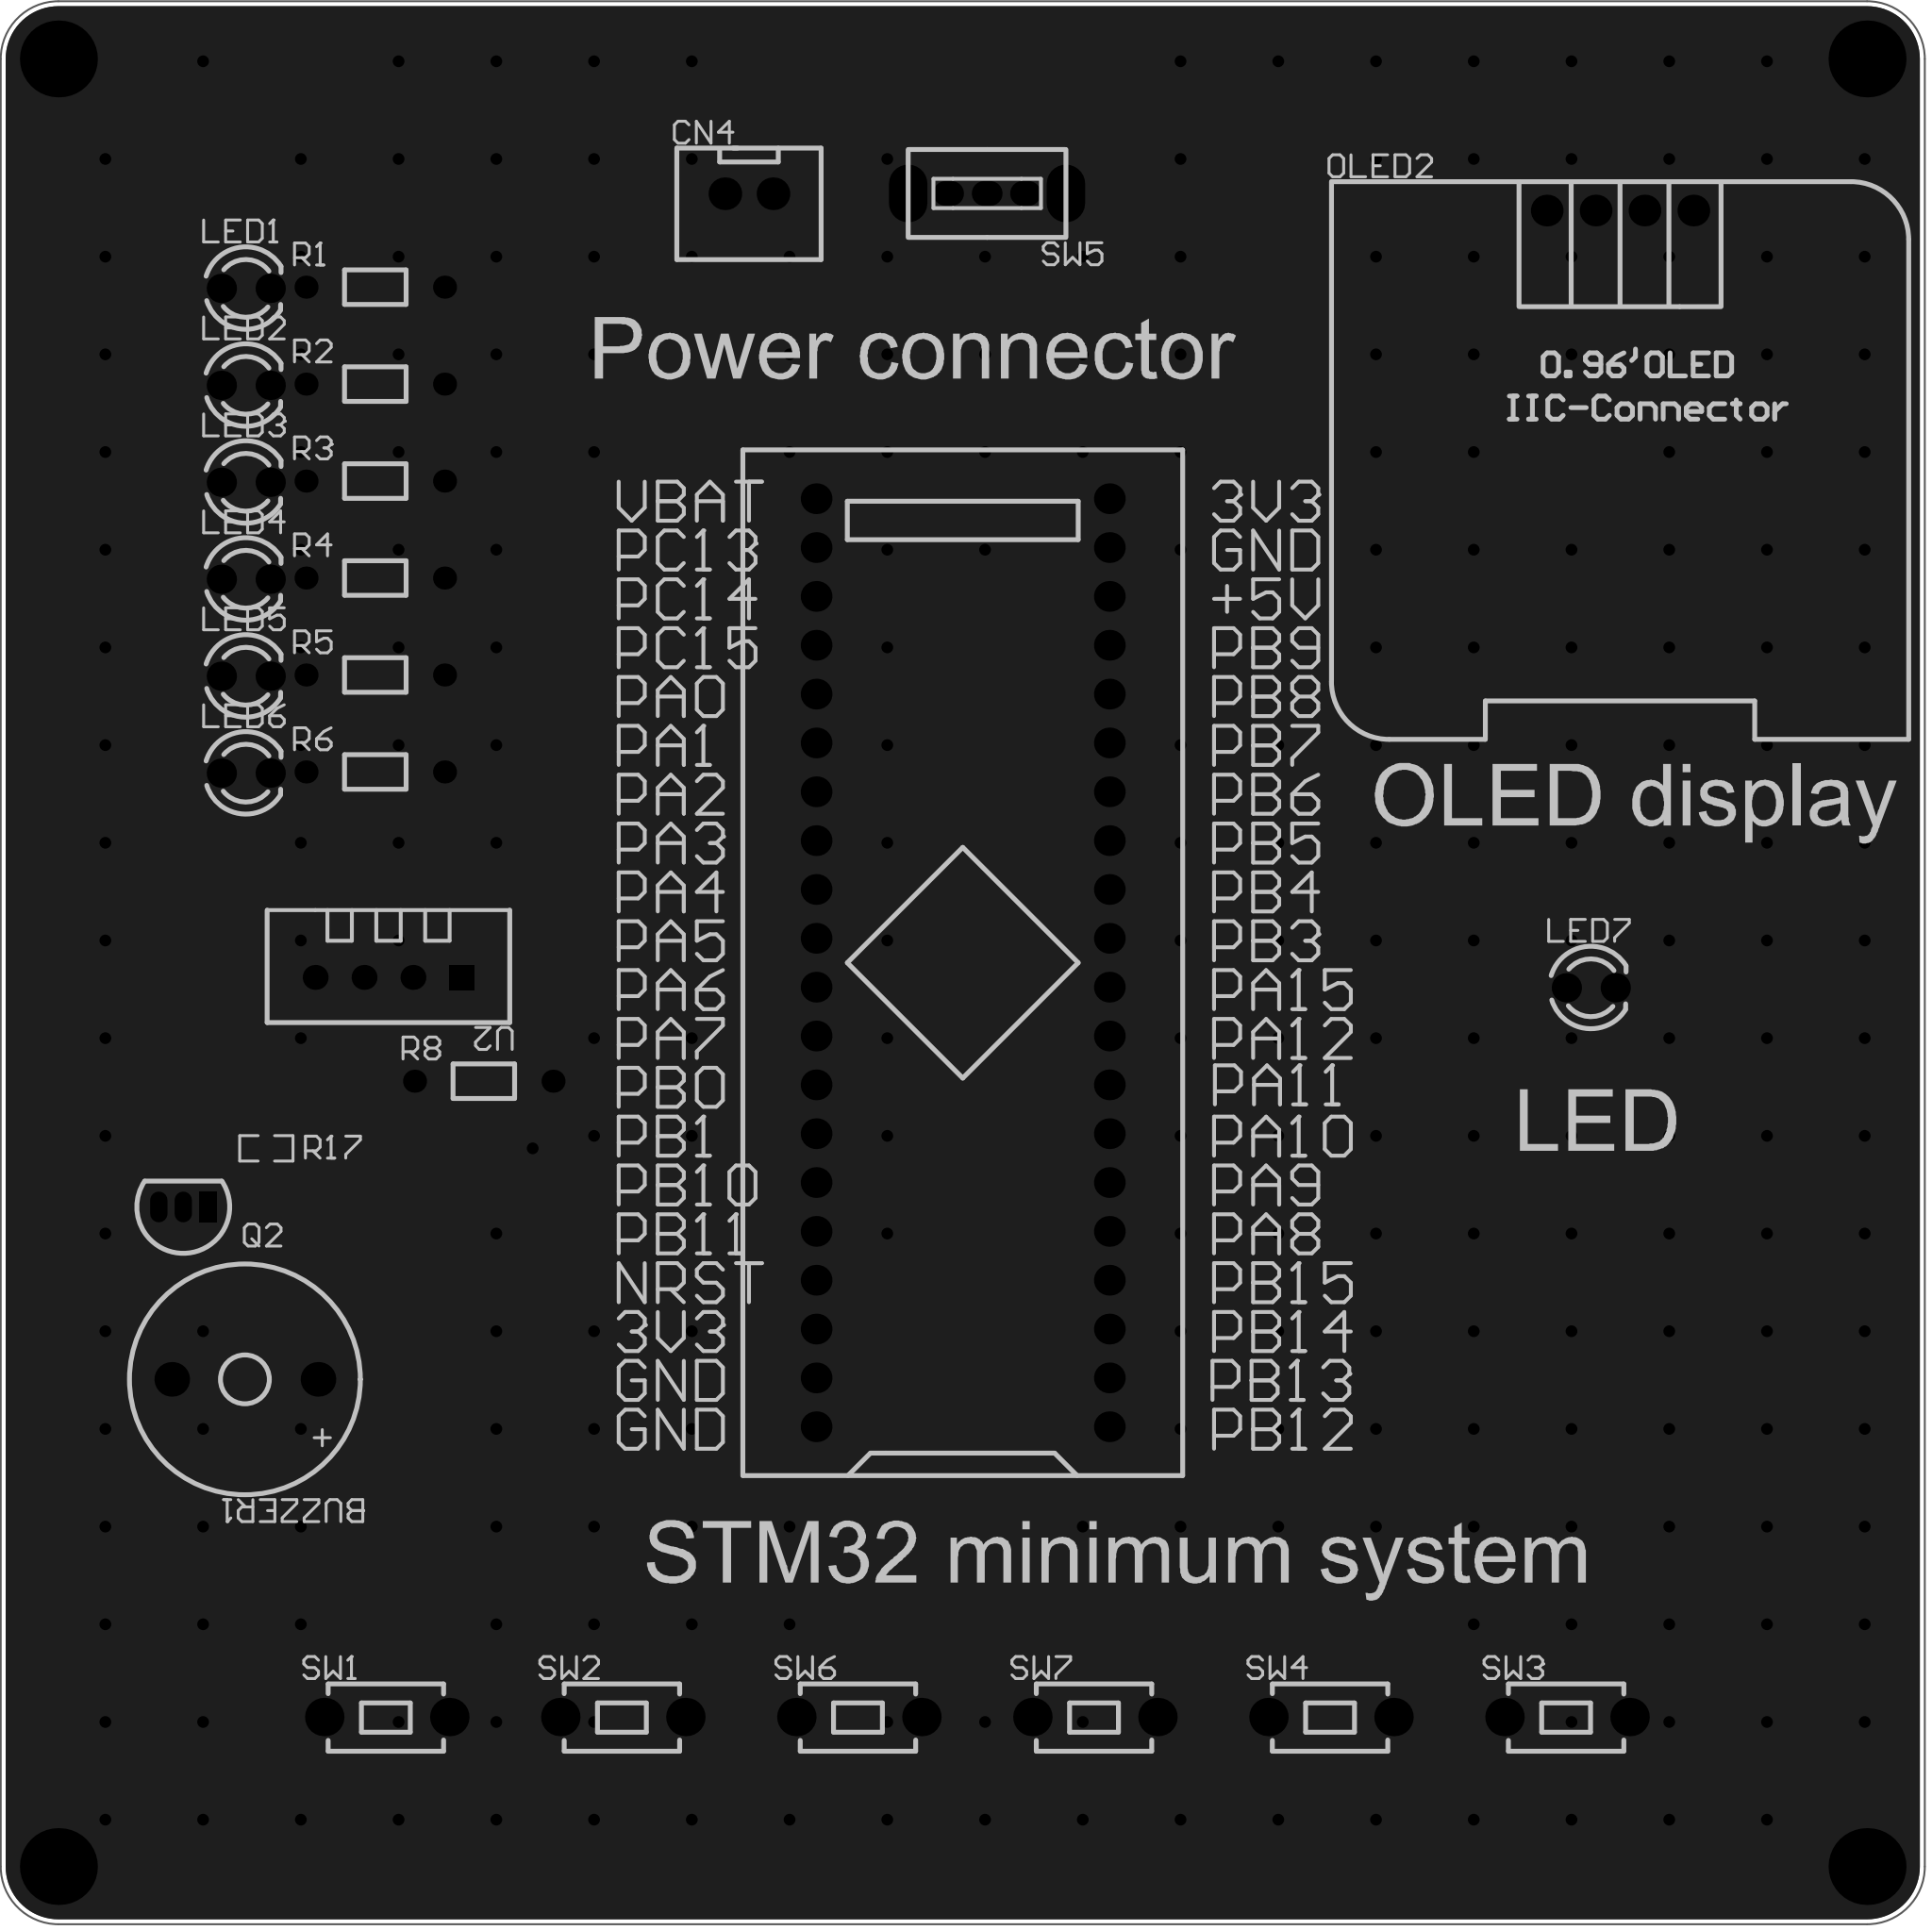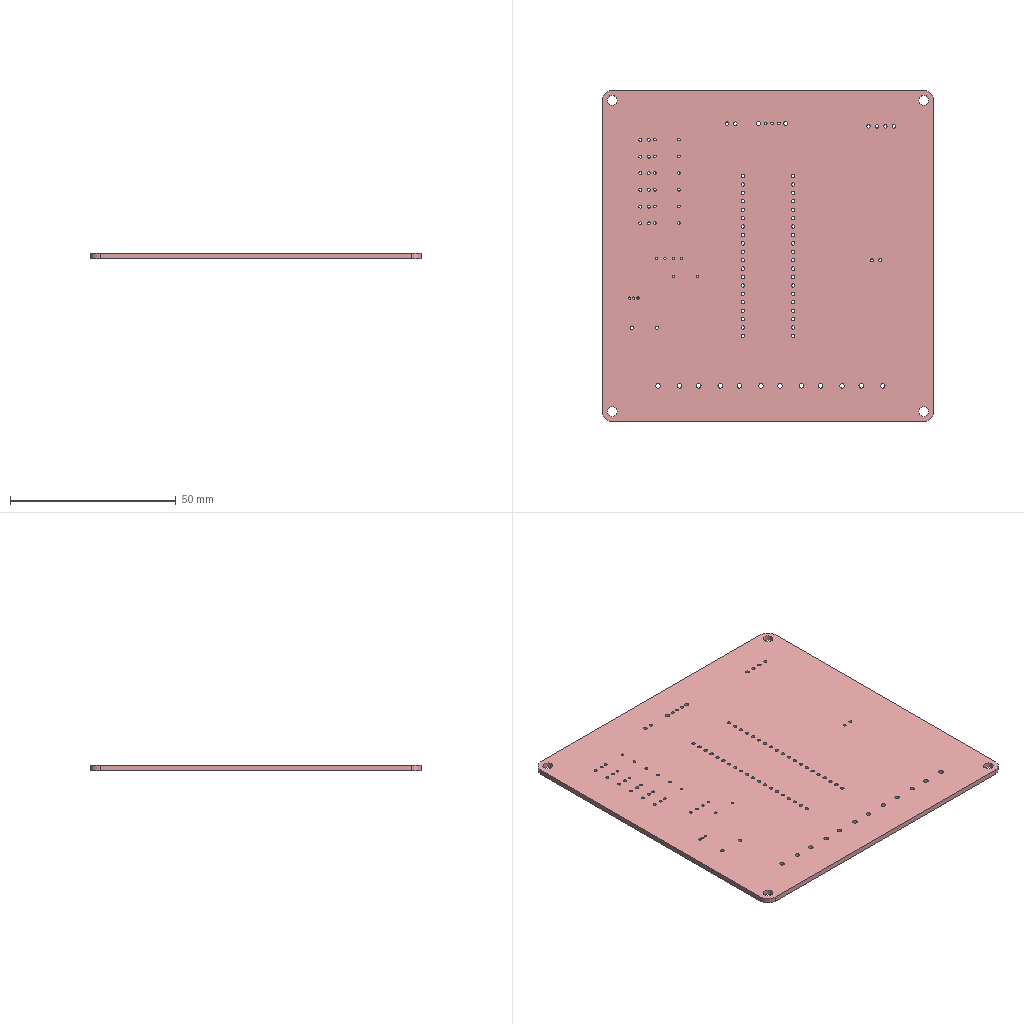Circuit board layout | Altium Designer | box 100 x 100 x 1.6 mm
Layer stack:
# Altium Designer layer stack of  (unit mm; dielectric type: 0 none, 1 core, 2 prepreg, 3 surface material)
index,name,kind,layer,copper_thickness_mm,dielectric_type,dielectric_thickness_mm,dielectric_material,dielectric_constant
0,Top Paste Mask Layer,other,,,,,,
1,Top Silkscreen Layer,other,,,,,,
2,Top Solder Mask Layer,dielectric,,,3,0.01,,3.3
3,Top Layer,copper,Top Layer,0.035,,,,
4,Dielectric1,dielectric,,,3,1.51,FR4,4.5
5,Bottom Layer,copper,Bottom Layer,0.035,,,,
6,Bottom Solder Mask Layer,dielectric,,,3,0.01,,3.3
7,Bottom Silkscreen Layer,other,,,,,,
8,Bottom Paste Mask Layer,other,,,,,,
# drill layer pairs: low layer,high layer
drill_pair,Top Layer,Bottom Layer
Part placement:
Designator,Comment,Layer,Footprint,Center-X(mm),Center-Y(mm),Rotation
U1,STM32F103C8T6-Card,TopLayer,CONN-TH_L53.3-W22.9_STM32F103C8T6-CARD,141.351,130.937,90
OLED2,,TopLayer,0.96OLED_4P,175.514,170.053,0
BUZZER1,2.4kHz,TopLayer,BUZ-TH_BD12.0-P7.60-D0.6-FD,104.041,109.272,180
LED1,,TopLayer,LED_TH-3mm,104.089,166.006,0
LED2,,TopLayer,LED_TH-3mm,104.089,160.964,0
LED3,,TopLayer,LED_TH-3mm,104.089,155.922,0
LED4,,TopLayer,LED_TH-3mm,104.089,150.88,0
LED5,,TopLayer,LED_TH-3mm,104.089,145.838,0
LED6,,TopLayer,LED_TH-3mm,104.089,140.796,0
R1,220Ω,TopLayer,Res_1/8W,110.82,166.069,0
R2,220Ω,TopLayer,Res_1/8W,110.82,161.027,0
R3,220Ω,TopLayer,Res_1/8W,110.82,155.985,0
R4,220Ω,TopLayer,Res_1/8W,110.82,150.943,0
R5,220Ω,TopLayer,Res_1/8W,110.82,145.901,0
R6,220Ω,TopLayer,Res_1/8W,110.82,140.859,0
R17,1kΩ,TopLayer,R0603,105.156,121.285,180
SW2,,TopLayer,Key_TH_3.5x6x4.3,123.686,91.712,0
SW3,,TopLayer,Key_TH_3.5x6x4.3,172.758,91.712,0
SW4,,TopLayer,Key_TH_3.5x6x4.3,160.49,91.712,0
SW7,,TopLayer,Key_TH_3.5x6x4.3,148.222,91.712,0
SW6,,TopLayer,Key_TH_3.5x6x4.3,135.954,91.712,0
SW1,,TopLayer,Key_TH_3.5x6x4.3,111.417,91.712,0
CN4,XH2.54*2P_through-hole,TopLayer,CONN-TH_2P-P2.50-XH2.54-2P,130.239,170.927,0
SW5,,TopLayer,拨动开关,142.613,170.942,180
LED7,,TopLayer,LED_TH-3mm,173.995,129.635,0
R8,4.7kΩ,TopLayer,Res_1/8W,116.459,124.777,0
U2,DHT11,TopLayer,SENSOR-TH_DHT11,111.506,130.175,180
Q2,,TopLayer,S8050_TO_92,100.838,118.237,180
Pad and via stacks:
# Altium Designer via and pad stacks of  (unit mm). Each distinct definition once, with the count of objects using it.
# via: kind,start_layer,end_layer,hole_mm,diameter_mm,mode(0 simple;1 top-mid-bottom;2 full stack),diameter_per_layer,count,example_net
# pad: kind,layer,hole_mm,hole_type(0 round;1 square;2 slot),plating,top_size,top_shape(1 round;2 rect;3 octagon;9 rounded rect),mid_size,bottom_size,mode,footprint,size_per_layer,count,example
pad,Multi-Layer,3,0,plated,4x4,1,4x4,4x4,0,,,4,1
pad,Multi-Layer,1,0,plated,1.6x1.6,1,1.6x1.6,1.6x1.6,0,CONN-TH_L53.3-W22.9_STM32F103C8T6-CARD,,40,U1.1
pad,Multi-Layer,1,0,plated,1.65x1.65,1,1.65x1.65,1.65x1.65,0,0.96OLED_4P,,4,OLED2.4
pad,Multi-Layer,1,0,plated,1.8x1.8,1,1.8x1.8,1.8x1.8,0,BUZ-TH_BD12.0-P7.60-D0.6-FD,,2,BUZZER1.2
pad,Multi-Layer,0.9144,0,plated,1.524x1.524,1,1.524x1.524,1.524x1.524,0,LED_TH-3mm,,14,LED1.1
pad,Multi-Layer,0.8001,0,plated,1.199x1.199,1,1.199x1.199,1.199x1.199,0,Res_1/8W,,14,R1.1
pad,Multi-Layer,1.399,0,plated,1.999x1.999,1,1.999x1.999,1.999x1.999,0,Key_TH_3.5x6x4.3,,12,SW2.A
pad,Multi-Layer,1.05,0,plated,1.7x1.7,1,1.7x1.7,1.7x1.7,0,CONN-TH_2P-P2.50-XH2.54-2P,,2,CN4.2
pad,Multi-Layer,0.8992,0,plated,1.6x1.3,1,1.6x1.3,1.6x1.3,0,\u00B2\u00A6\u00B6\u00AF\u00BF\u00AA\u00B9\u00D8,,3,SW5.1
pad,Multi-Layer,1.3,0,plated,3x1.999,1,3x1.999,3x1.999,0,\u00B2\u00A6\u00B6\u00AF\u00BF\u00AA\u00B9\u00D8,,2,SW5.4
pad,Multi-Layer,0.7112,0,plated,1.295x1.295,2,1.295x1.295,1.295x1.295,0,SENSOR-TH_DHT11,,1,U2.1
pad,Multi-Layer,0.7112,0,plated,1.295x1.295,1,1.295x1.295,1.295x1.295,0,SENSOR-TH_DHT11,,3,U2.2
pad,Multi-Layer,0.701,0,plated,0.8992x1.6,2,0.8992x1.6,0.8992x1.6,0,S8050_TO_92,,1,Q2.1
pad,Multi-Layer,0.701,0,plated,0.8992x1.6,1,0.8992x1.6,0.8992x1.6,0,S8050_TO_92,,2,Q2.2
pad,Top Layer,0,0,plated,0.8065x0.864,2,0.8065x0.864,0.8065x0.864,0,R0603,,2,R17.2
via,Top Layer,Bottom Layer,0.3048,0.61,0,,258,PA8
Copper pours:
name,layer,net,type(0 solid;1 hatched;2 none)
Bottom Layer-GND,Bottom Layer,GND,0
Top Layer-GND,Top Layer,GND,0
Design rules, without the lines most boards share:
# Altium Designer design rules of  (exported by Altium Designer, unit mm)
# columns: name | kind | enabled | priority | scope1 | scope2 | descriptor | typed fields (field=value)
Copper_copperRegion_copperThickness1oz | 0 | disabled | 4 | All | All | Clearance Constraint (Gap=5.984mil) (Disabled)(All),(All) | gap=0.152
Copper_copperRegion_copperThickness1oz_1 | 63 | disabled | 4 | All | All | Board Clearance Constraint (Gap=0mil) (Disabled)(All) |
Copper_copperRegion_Copper_copperRegion | 0 | disabled | 5 | All | All | Clearance Constraint (Gap=5.984mil) (Disabled)(All),(All) | gap=0.152
Copper_copperRegion_Copper_copperRegion_1 | 63 | disabled | 5 | All | All | Board Clearance Constraint (Gap=0mil) (Disabled)(All) |
copperThickness1oz | 0 | enabled | 6 | All | All | Clearance Constraint (Gap=5.984mil) (All),(All) | gap=0.152
copperThickness1oz_1 | 63 | enabled | 6 | All | All | Board Clearance Constraint (Gap=0mil) (All) |
copperRegion_copperThickness1oz | 20 | disabled | 1 | All | All | Polygon Connect Rule(Relief Connect )(Conductor Width=10mil) (Relief Angle=90 Angle) (Entries=4) (Air Gap Width=10mil) (Disabled)(All),(All) | connect_style(0=relief,1=direct,2=none)=0 relief_conductor_width=0.254 relief_entries=4
copperRegion_Copper_copperRegion | 20 | disabled | 2 | All | All | Polygon Connect Rule(Relief Connect )(Conductor Width=10mil) (Relief Angle=90 Angle) (Entries=4) (Air Gap Width=10mil) (Disabled)(All),(All) | connect_style(0=relief,1=direct,2=none)=0 relief_conductor_width=0.254 relief_entries=4
copperRegion | 20 | enabled | 3 | All | All | Polygon Connect Rule(Relief Connect )(Conductor Width=10mil) (Relief Angle=90 Angle) (Entries=4) (Air Gap Width=10mil) (All),(All) | connect_style(0=relief,1=direct,2=none)=0 relief_conductor_width=0.254 relief_entries=4